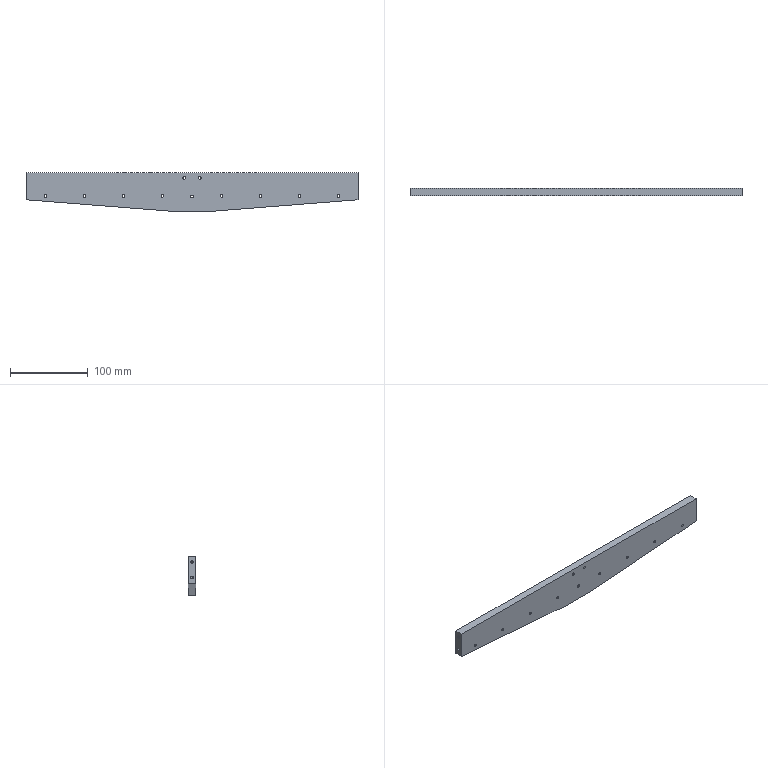Part | SolidWorks | features HoleWzd 3, Chamfer 2, MirrorPattern 2, Extrusion 1 | 1 solid | 55 faces | box 426 x 10 x 50 mm | volume 182893 mm3 | cylinder 36 | plane 11 | cone 8 | commonest cylinder face diameters 3.3 x24 3.4 x6 6.5 x6